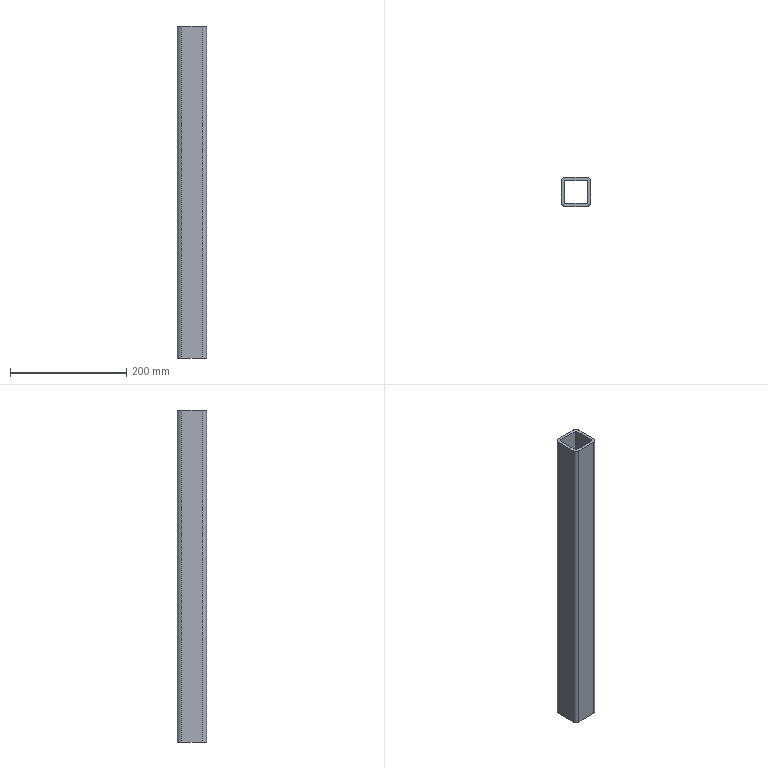Part | NX | 1 solid | 18 faces | box 50 x 50 x 570 mm | volume 490982 mm3 | plane 10 | cylinder 8 | commonest cylinder face diameters 4 x4 14 x4
STEP:
#1=CARTESIAN_POINT('',(-645.,-18.,285.));
#2=VERTEX_POINT('',#1);
#3=CARTESIAN_POINT('',(-645.,-18.,-285.));
#4=VERTEX_POINT('',#3);
#5=CARTESIAN_POINT('',(-645.,-18.,310.));
#6=DIRECTION('',(0.,0.,-1.));
#7=VECTOR('',#6,1000.);
#8=LINE('',#5,#7);
#9=EDGE_CURVE('',#2,#4,#8,.T.);
#10=ORIENTED_EDGE('',*,*,#9,.T.);
#11=CARTESIAN_POINT('',(-645.,18.,-285.));
#12=VERTEX_POINT('',#11);
#13=CARTESIAN_POINT('',(-645.,-18.,-285.));
#14=DIRECTION('',(0.,1.,0.));
#15=VECTOR('',#14,1000.);
#16=LINE('',#13,#15);
#17=EDGE_CURVE('',#4,#12,#16,.T.);
#18=ORIENTED_EDGE('',*,*,#17,.T.);
#19=CARTESIAN_POINT('',(-645.,18.,285.));
#20=VERTEX_POINT('',#19);
#21=CARTESIAN_POINT('',(-645.,18.,310.));
#22=DIRECTION('',(0.,0.,-1.));
#23=VECTOR('',#22,1000.);
#24=LINE('',#21,#23);
#25=EDGE_CURVE('',#20,#12,#24,.T.);
#26=ORIENTED_EDGE('',*,*,#25,.F.);
#27=CARTESIAN_POINT('',(-645.,-18.,285.));
#28=DIRECTION('',(0.,-1.,0.));
#29=VECTOR('',#28,1000.);
#30=LINE('',#27,#29);
#31=EDGE_CURVE('',#20,#2,#30,.T.);
#32=ORIENTED_EDGE('',*,*,#31,.T.);
#33=EDGE_LOOP('',(#10,#18,#26,#32));
#34=FACE_BOUND('',#33,.T.);
#35=CARTESIAN_POINT('',(-645.,-18.,310.));
#36=DIRECTION('',(1.,0.,0.));
#37=DIRECTION('',(0.,1.,0.));
#38=AXIS2_PLACEMENT_3D('',#35,#36,#37);
#39=PLANE('',#38);
#40=ADVANCED_FACE('',(#34),#39,.T.);
#41=CARTESIAN_POINT('',(-643.,-20.,285.));
#42=VERTEX_POINT('',#41);
#43=CARTESIAN_POINT('',(-643.,-20.,-285.));
#44=VERTEX_POINT('',#43);
#45=CARTESIAN_POINT('',(-643.,-20.,310.));
#46=DIRECTION('',(0.,0.,-1.));
#47=VECTOR('',#46,1000.);
#48=LINE('',#45,#47);
#49=EDGE_CURVE('',#42,#44,#48,.T.);
#50=ORIENTED_EDGE('',*,*,#49,.T.);
#51=CARTESIAN_POINT('',(-643.,-18.,-285.));
#52=DIRECTION('',(0.,0.,-1.));
#53=DIRECTION('',(-1.,0.,0.));
#54=AXIS2_PLACEMENT_3D('',#51,#52,#53);
#55=CIRCLE('',#54,2.);
#56=EDGE_CURVE('',#44,#4,#55,.T.);
#57=ORIENTED_EDGE('',*,*,#56,.T.);
#58=ORIENTED_EDGE('',*,*,#9,.F.);
#59=CARTESIAN_POINT('',(-643.,-18.,285.));
#60=DIRECTION('',(0.,0.,1.));
#61=DIRECTION('',(1.,0.,0.));
#62=AXIS2_PLACEMENT_3D('',#59,#60,#61);
#63=CIRCLE('',#62,2.);
#64=EDGE_CURVE('',#2,#42,#63,.T.);
#65=ORIENTED_EDGE('',*,*,#64,.T.);
#66=EDGE_LOOP('',(#50,#57,#58,#65));
#67=FACE_BOUND('',#66,.T.);
#68=CARTESIAN_POINT('',(-643.,-18.,310.));
#69=DIRECTION('',(0.,0.,-1.));
#70=DIRECTION('',(-1.,0.,0.));
#71=AXIS2_PLACEMENT_3D('',#68,#69,#70);
#72=CYLINDRICAL_SURFACE('',#71,2.);
#73=ADVANCED_FACE('',(#67),#72,.F.);
#74=CARTESIAN_POINT('',(-607.,-20.,285.));
#75=VERTEX_POINT('',#74);
#76=CARTESIAN_POINT('',(-607.,-20.,-285.));
#77=VERTEX_POINT('',#76);
#78=CARTESIAN_POINT('',(-607.,-20.,310.));
#79=DIRECTION('',(0.,0.,-1.));
#80=VECTOR('',#79,1000.);
#81=LINE('',#78,#80);
#82=EDGE_CURVE('',#75,#77,#81,.T.);
#83=ORIENTED_EDGE('',*,*,#82,.T.);
#84=CARTESIAN_POINT('',(-643.,-20.,-285.));
#85=DIRECTION('',(-1.,0.,0.));
#86=VECTOR('',#85,1000.);
#87=LINE('',#84,#86);
#88=EDGE_CURVE('',#77,#44,#87,.T.);
#89=ORIENTED_EDGE('',*,*,#88,.T.);
#90=ORIENTED_EDGE('',*,*,#49,.F.);
#91=CARTESIAN_POINT('',(-643.,-20.,285.));
#92=DIRECTION('',(1.,0.,0.));
#93=VECTOR('',#92,1000.);
#94=LINE('',#91,#93);
#95=EDGE_CURVE('',#42,#75,#94,.T.);
#96=ORIENTED_EDGE('',*,*,#95,.T.);
#97=EDGE_LOOP('',(#83,#89,#90,#96));
#98=FACE_BOUND('',#97,.T.);
#99=CARTESIAN_POINT('',(-643.,-20.,310.));
#100=DIRECTION('',(0.,1.,0.));
#101=DIRECTION('',(-1.,0.,0.));
#102=AXIS2_PLACEMENT_3D('',#99,#100,#101);
#103=PLANE('',#102);
#104=ADVANCED_FACE('',(#98),#103,.T.);
#105=CARTESIAN_POINT('',(-605.,-18.,285.));
#106=VERTEX_POINT('',#105);
#107=CARTESIAN_POINT('',(-605.,-18.,-285.));
#108=VERTEX_POINT('',#107);
#109=CARTESIAN_POINT('',(-605.,-18.,310.));
#110=DIRECTION('',(0.,0.,-1.));
#111=VECTOR('',#110,1000.);
#112=LINE('',#109,#111);
#113=EDGE_CURVE('',#106,#108,#112,.T.);
#114=ORIENTED_EDGE('',*,*,#113,.T.);
#115=CARTESIAN_POINT('',(-607.,-18.,-285.));
#116=DIRECTION('',(0.,0.,-1.));
#117=DIRECTION('',(-1.,0.,0.));
#118=AXIS2_PLACEMENT_3D('',#115,#116,#117);
#119=CIRCLE('',#118,2.);
#120=EDGE_CURVE('',#108,#77,#119,.T.);
#121=ORIENTED_EDGE('',*,*,#120,.T.);
#122=ORIENTED_EDGE('',*,*,#82,.F.);
#123=CARTESIAN_POINT('',(-607.,-18.,285.));
#124=DIRECTION('',(0.,0.,1.));
#125=DIRECTION('',(1.,0.,0.));
#126=AXIS2_PLACEMENT_3D('',#123,#124,#125);
#127=CIRCLE('',#126,2.);
#128=EDGE_CURVE('',#75,#106,#127,.T.);
#129=ORIENTED_EDGE('',*,*,#128,.T.);
#130=EDGE_LOOP('',(#114,#121,#122,#129));
#131=FACE_BOUND('',#130,.T.);
#132=CARTESIAN_POINT('',(-607.,-18.,310.));
#133=DIRECTION('',(0.,0.,-1.));
#134=DIRECTION('',(-1.,0.,0.));
#135=AXIS2_PLACEMENT_3D('',#132,#133,#134);
#136=CYLINDRICAL_SURFACE('',#135,2.);
#137=ADVANCED_FACE('',(#131),#136,.F.);
#138=CARTESIAN_POINT('',(-605.,18.,285.));
#139=VERTEX_POINT('',#138);
#140=CARTESIAN_POINT('',(-605.,18.,-285.));
#141=VERTEX_POINT('',#140);
#142=CARTESIAN_POINT('',(-605.,18.,310.));
#143=DIRECTION('',(0.,0.,-1.));
#144=VECTOR('',#143,1000.);
#145=LINE('',#142,#144);
#146=EDGE_CURVE('',#139,#141,#145,.T.);
#147=ORIENTED_EDGE('',*,*,#146,.T.);
#148=CARTESIAN_POINT('',(-605.,18.,-285.));
#149=DIRECTION('',(0.,-1.,0.));
#150=VECTOR('',#149,1000.);
#151=LINE('',#148,#150);
#152=EDGE_CURVE('',#141,#108,#151,.T.);
#153=ORIENTED_EDGE('',*,*,#152,.T.);
#154=ORIENTED_EDGE('',*,*,#113,.F.);
#155=CARTESIAN_POINT('',(-605.,18.,285.));
#156=DIRECTION('',(0.,1.,0.));
#157=VECTOR('',#156,1000.);
#158=LINE('',#155,#157);
#159=EDGE_CURVE('',#106,#139,#158,.T.);
#160=ORIENTED_EDGE('',*,*,#159,.T.);
#161=EDGE_LOOP('',(#147,#153,#154,#160));
#162=FACE_BOUND('',#161,.T.);
#163=CARTESIAN_POINT('',(-605.,18.,310.));
#164=DIRECTION('',(-1.,0.,0.));
#165=DIRECTION('',(0.,-1.,0.));
#166=AXIS2_PLACEMENT_3D('',#163,#164,#165);
#167=PLANE('',#166);
#168=ADVANCED_FACE('',(#162),#167,.T.);
#169=CARTESIAN_POINT('',(-607.,20.,285.));
#170=VERTEX_POINT('',#169);
#171=CARTESIAN_POINT('',(-607.,20.,-285.));
#172=VERTEX_POINT('',#171);
#173=CARTESIAN_POINT('',(-607.,20.,310.));
#174=DIRECTION('',(0.,0.,-1.));
#175=VECTOR('',#174,1000.);
#176=LINE('',#173,#175);
#177=EDGE_CURVE('',#170,#172,#176,.T.);
#178=ORIENTED_EDGE('',*,*,#177,.T.);
#179=CARTESIAN_POINT('',(-607.,18.,-285.));
#180=DIRECTION('',(0.,0.,-1.));
#181=DIRECTION('',(-1.,0.,0.));
#182=AXIS2_PLACEMENT_3D('',#179,#180,#181);
#183=CIRCLE('',#182,2.);
#184=EDGE_CURVE('',#172,#141,#183,.T.);
#185=ORIENTED_EDGE('',*,*,#184,.T.);
#186=ORIENTED_EDGE('',*,*,#146,.F.);
#187=CARTESIAN_POINT('',(-607.,18.,285.));
#188=DIRECTION('',(0.,0.,1.));
#189=DIRECTION('',(1.,0.,0.));
#190=AXIS2_PLACEMENT_3D('',#187,#188,#189);
#191=CIRCLE('',#190,2.);
#192=EDGE_CURVE('',#139,#170,#191,.T.);
#193=ORIENTED_EDGE('',*,*,#192,.T.);
#194=EDGE_LOOP('',(#178,#185,#186,#193));
#195=FACE_BOUND('',#194,.T.);
#196=CARTESIAN_POINT('',(-607.,18.,310.));
#197=DIRECTION('',(0.,0.,-1.));
#198=DIRECTION('',(-1.,0.,0.));
#199=AXIS2_PLACEMENT_3D('',#196,#197,#198);
#200=CYLINDRICAL_SURFACE('',#199,2.);
#201=ADVANCED_FACE('',(#195),#200,.F.);
#202=CARTESIAN_POINT('',(-643.,20.,285.));
#203=VERTEX_POINT('',#202);
#204=CARTESIAN_POINT('',(-643.,20.,-285.));
#205=VERTEX_POINT('',#204);
#206=CARTESIAN_POINT('',(-643.,20.,310.));
#207=DIRECTION('',(0.,0.,-1.));
#208=VECTOR('',#207,1000.);
#209=LINE('',#206,#208);
#210=EDGE_CURVE('',#203,#205,#209,.T.);
#211=ORIENTED_EDGE('',*,*,#210,.T.);
#212=CARTESIAN_POINT('',(-607.,20.,-285.));
#213=DIRECTION('',(1.,0.,0.));
#214=VECTOR('',#213,1000.);
#215=LINE('',#212,#214);
#216=EDGE_CURVE('',#205,#172,#215,.T.);
#217=ORIENTED_EDGE('',*,*,#216,.T.);
#218=ORIENTED_EDGE('',*,*,#177,.F.);
#219=CARTESIAN_POINT('',(-607.,20.,285.));
#220=DIRECTION('',(-1.,0.,0.));
#221=VECTOR('',#220,1000.);
#222=LINE('',#219,#221);
#223=EDGE_CURVE('',#170,#203,#222,.T.);
#224=ORIENTED_EDGE('',*,*,#223,.T.);
#225=EDGE_LOOP('',(#211,#217,#218,#224));
#226=FACE_BOUND('',#225,.T.);
#227=CARTESIAN_POINT('',(-607.,20.,310.));
#228=DIRECTION('',(0.,-1.,0.));
#229=DIRECTION('',(1.,0.,0.));
#230=AXIS2_PLACEMENT_3D('',#227,#228,#229);
#231=PLANE('',#230);
#232=ADVANCED_FACE('',(#226),#231,.T.);
#233=ORIENTED_EDGE('',*,*,#25,.T.);
#234=CARTESIAN_POINT('',(-643.,18.,-285.));
#235=DIRECTION('',(0.,0.,-1.));
#236=DIRECTION('',(-1.,0.,0.));
#237=AXIS2_PLACEMENT_3D('',#234,#235,#236);
#238=CIRCLE('',#237,2.);
#239=EDGE_CURVE('',#12,#205,#238,.T.);
#240=ORIENTED_EDGE('',*,*,#239,.T.);
#241=ORIENTED_EDGE('',*,*,#210,.F.);
#242=CARTESIAN_POINT('',(-643.,18.,285.));
#243=DIRECTION('',(0.,0.,1.));
#244=DIRECTION('',(1.,0.,0.));
#245=AXIS2_PLACEMENT_3D('',#242,#243,#244);
#246=CIRCLE('',#245,2.);
#247=EDGE_CURVE('',#203,#20,#246,.T.);
#248=ORIENTED_EDGE('',*,*,#247,.T.);
#249=EDGE_LOOP('',(#233,#240,#241,#248));
#250=FACE_BOUND('',#249,.T.);
#251=CARTESIAN_POINT('',(-643.,18.,310.));
#252=DIRECTION('',(0.,0.,-1.));
#253=DIRECTION('',(-1.,0.,0.));
#254=AXIS2_PLACEMENT_3D('',#251,#252,#253);
#255=CYLINDRICAL_SURFACE('',#254,2.);
#256=ADVANCED_FACE('',(#250),#255,.F.);
#257=CARTESIAN_POINT('',(-600.,18.,-285.));
#258=VERTEX_POINT('',#257);
#259=CARTESIAN_POINT('',(-600.,-18.,-285.));
#260=VERTEX_POINT('',#259);
#261=CARTESIAN_POINT('',(-600.,18.,-285.));
#262=DIRECTION('',(0.,-1.,0.));
#263=VECTOR('',#262,1000.);
#264=LINE('',#261,#263);
#265=EDGE_CURVE('',#258,#260,#264,.T.);
#266=ORIENTED_EDGE('',*,*,#265,.F.);
#267=CARTESIAN_POINT('',(-600.,18.,285.));
#268=VERTEX_POINT('',#267);
#269=CARTESIAN_POINT('',(-600.,18.,310.));
#270=DIRECTION('',(0.,0.,-1.));
#271=VECTOR('',#270,1000.);
#272=LINE('',#269,#271);
#273=EDGE_CURVE('',#268,#258,#272,.T.);
#274=ORIENTED_EDGE('',*,*,#273,.F.);
#275=CARTESIAN_POINT('',(-600.,-18.,285.));
#276=VERTEX_POINT('',#275);
#277=CARTESIAN_POINT('',(-600.,18.,285.));
#278=DIRECTION('',(0.,1.,0.));
#279=VECTOR('',#278,1000.);
#280=LINE('',#277,#279);
#281=EDGE_CURVE('',#276,#268,#280,.T.);
#282=ORIENTED_EDGE('',*,*,#281,.F.);
#283=CARTESIAN_POINT('',(-600.,-18.,310.));
#284=DIRECTION('',(0.,0.,-1.));
#285=VECTOR('',#284,1000.);
#286=LINE('',#283,#285);
#287=EDGE_CURVE('',#276,#260,#286,.T.);
#288=ORIENTED_EDGE('',*,*,#287,.T.);
#289=EDGE_LOOP('',(#266,#274,#282,#288));
#290=FACE_BOUND('',#289,.T.);
#291=CARTESIAN_POINT('',(-600.,18.,310.));
#292=DIRECTION('',(-1.,0.,0.));
#293=DIRECTION('',(0.,-1.,0.));
#294=AXIS2_PLACEMENT_3D('',#291,#292,#293);
#295=PLANE('',#294);
#296=ADVANCED_FACE('',(#290),#295,.F.);
#297=CARTESIAN_POINT('',(-607.,-25.,-285.));
#298=VERTEX_POINT('',#297);
#299=CARTESIAN_POINT('',(-607.,-18.,-285.));
#300=DIRECTION('',(0.,0.,-1.));
#301=DIRECTION('',(-1.,0.,0.));
#302=AXIS2_PLACEMENT_3D('',#299,#300,#301);
#303=CIRCLE('',#302,7.);
#304=EDGE_CURVE('',#260,#298,#303,.T.);
#305=ORIENTED_EDGE('',*,*,#304,.F.);
#306=ORIENTED_EDGE('',*,*,#287,.F.);
#307=CARTESIAN_POINT('',(-607.,-25.,285.));
#308=VERTEX_POINT('',#307);
#309=CARTESIAN_POINT('',(-607.,-18.,285.));
#310=DIRECTION('',(0.,0.,1.));
#311=DIRECTION('',(1.,0.,0.));
#312=AXIS2_PLACEMENT_3D('',#309,#310,#311);
#313=CIRCLE('',#312,7.);
#314=EDGE_CURVE('',#308,#276,#313,.T.);
#315=ORIENTED_EDGE('',*,*,#314,.F.);
#316=CARTESIAN_POINT('',(-607.,-25.,310.));
#317=DIRECTION('',(0.,0.,-1.));
#318=VECTOR('',#317,1000.);
#319=LINE('',#316,#318);
#320=EDGE_CURVE('',#308,#298,#319,.T.);
#321=ORIENTED_EDGE('',*,*,#320,.T.);
#322=EDGE_LOOP('',(#305,#306,#315,#321));
#323=FACE_BOUND('',#322,.T.);
#324=CARTESIAN_POINT('',(-607.,-18.,310.));
#325=DIRECTION('',(0.,0.,-1.));
#326=DIRECTION('',(-1.,0.,0.));
#327=AXIS2_PLACEMENT_3D('',#324,#325,#326);
#328=CYLINDRICAL_SURFACE('',#327,7.);
#329=ADVANCED_FACE('',(#323),#328,.T.);
#330=CARTESIAN_POINT('',(-643.,-25.,-285.));
#331=VERTEX_POINT('',#330);
#332=CARTESIAN_POINT('',(-875.,-25.,-285.));
#333=DIRECTION('',(1.,0.,0.));
#334=VECTOR('',#333,1000.);
#335=LINE('',#332,#334);
#336=EDGE_CURVE('',#331,#298,#335,.T.);
#337=ORIENTED_EDGE('',*,*,#336,.T.);
#338=ORIENTED_EDGE('',*,*,#320,.F.);
#339=CARTESIAN_POINT('',(-643.,-25.,285.));
#340=VERTEX_POINT('',#339);
#341=CARTESIAN_POINT('',(-875.,-25.,285.));
#342=DIRECTION('',(1.,0.,0.));
#343=VECTOR('',#342,1000.);
#344=LINE('',#341,#343);
#345=EDGE_CURVE('',#340,#308,#344,.T.);
#346=ORIENTED_EDGE('',*,*,#345,.F.);
#347=CARTESIAN_POINT('',(-643.,-25.,310.));
#348=DIRECTION('',(0.,0.,-1.));
#349=VECTOR('',#348,1000.);
#350=LINE('',#347,#349);
#351=EDGE_CURVE('',#340,#331,#350,.T.);
#352=ORIENTED_EDGE('',*,*,#351,.T.);
#353=EDGE_LOOP('',(#337,#338,#346,#352));
#354=FACE_BOUND('',#353,.T.);
#355=CARTESIAN_POINT('',(-643.,-25.,310.));
#356=DIRECTION('',(0.,1.,0.));
#357=DIRECTION('',(-1.,0.,0.));
#358=AXIS2_PLACEMENT_3D('',#355,#356,#357);
#359=PLANE('',#358);
#360=ADVANCED_FACE('',(#354),#359,.F.);
#361=CARTESIAN_POINT('',(-650.,-18.,-285.));
#362=VERTEX_POINT('',#361);
#363=CARTESIAN_POINT('',(-643.,-18.,-285.));
#364=DIRECTION('',(0.,0.,-1.));
#365=DIRECTION('',(-1.,0.,0.));
#366=AXIS2_PLACEMENT_3D('',#363,#364,#365);
#367=CIRCLE('',#366,7.);
#368=EDGE_CURVE('',#331,#362,#367,.T.);
#369=ORIENTED_EDGE('',*,*,#368,.F.);
#370=ORIENTED_EDGE('',*,*,#351,.F.);
#371=CARTESIAN_POINT('',(-650.,-18.,285.));
#372=VERTEX_POINT('',#371);
#373=CARTESIAN_POINT('',(-643.,-18.,285.));
#374=DIRECTION('',(0.,0.,1.));
#375=DIRECTION('',(1.,0.,0.));
#376=AXIS2_PLACEMENT_3D('',#373,#374,#375);
#377=CIRCLE('',#376,7.);
#378=EDGE_CURVE('',#372,#340,#377,.T.);
#379=ORIENTED_EDGE('',*,*,#378,.F.);
#380=CARTESIAN_POINT('',(-650.,-18.,310.));
#381=DIRECTION('',(0.,0.,-1.));
#382=VECTOR('',#381,1000.);
#383=LINE('',#380,#382);
#384=EDGE_CURVE('',#372,#362,#383,.T.);
#385=ORIENTED_EDGE('',*,*,#384,.T.);
#386=EDGE_LOOP('',(#369,#370,#379,#385));
#387=FACE_BOUND('',#386,.T.);
#388=CARTESIAN_POINT('',(-643.,-18.,310.));
#389=DIRECTION('',(0.,0.,-1.));
#390=DIRECTION('',(-1.,0.,0.));
#391=AXIS2_PLACEMENT_3D('',#388,#389,#390);
#392=CYLINDRICAL_SURFACE('',#391,7.);
#393=ADVANCED_FACE('',(#387),#392,.T.);
#394=CARTESIAN_POINT('',(-650.,18.,-285.));
#395=VERTEX_POINT('',#394);
#396=CARTESIAN_POINT('',(-650.,-18.,-285.));
#397=DIRECTION('',(0.,1.,0.));
#398=VECTOR('',#397,1000.);
#399=LINE('',#396,#398);
#400=EDGE_CURVE('',#362,#395,#399,.T.);
#401=ORIENTED_EDGE('',*,*,#400,.F.);
#402=ORIENTED_EDGE('',*,*,#384,.F.);
#403=CARTESIAN_POINT('',(-650.,18.,285.));
#404=VERTEX_POINT('',#403);
#405=CARTESIAN_POINT('',(-650.,-18.,285.));
#406=DIRECTION('',(0.,-1.,0.));
#407=VECTOR('',#406,1000.);
#408=LINE('',#405,#407);
#409=EDGE_CURVE('',#404,#372,#408,.T.);
#410=ORIENTED_EDGE('',*,*,#409,.F.);
#411=CARTESIAN_POINT('',(-650.,18.,310.));
#412=DIRECTION('',(0.,0.,-1.));
#413=VECTOR('',#412,1000.);
#414=LINE('',#411,#413);
#415=EDGE_CURVE('',#404,#395,#414,.T.);
#416=ORIENTED_EDGE('',*,*,#415,.T.);
#417=EDGE_LOOP('',(#401,#402,#410,#416));
#418=FACE_BOUND('',#417,.T.);
#419=CARTESIAN_POINT('',(-650.,-18.,310.));
#420=DIRECTION('',(1.,0.,0.));
#421=DIRECTION('',(0.,1.,0.));
#422=AXIS2_PLACEMENT_3D('',#419,#420,#421);
#423=PLANE('',#422);
#424=ADVANCED_FACE('',(#418),#423,.F.);
#425=CARTESIAN_POINT('',(-643.,25.,-285.));
#426=VERTEX_POINT('',#425);
#427=CARTESIAN_POINT('',(-643.,18.,-285.));
#428=DIRECTION('',(0.,0.,-1.));
#429=DIRECTION('',(-1.,0.,0.));
#430=AXIS2_PLACEMENT_3D('',#427,#428,#429);
#431=CIRCLE('',#430,7.);
#432=EDGE_CURVE('',#395,#426,#431,.T.);
#433=ORIENTED_EDGE('',*,*,#432,.F.);
#434=ORIENTED_EDGE('',*,*,#415,.F.);
#435=CARTESIAN_POINT('',(-643.,25.,285.));
#436=VERTEX_POINT('',#435);
#437=CARTESIAN_POINT('',(-643.,18.,285.));
#438=DIRECTION('',(0.,0.,1.));
#439=DIRECTION('',(1.,0.,0.));
#440=AXIS2_PLACEMENT_3D('',#437,#438,#439);
#441=CIRCLE('',#440,7.);
#442=EDGE_CURVE('',#436,#404,#441,.T.);
#443=ORIENTED_EDGE('',*,*,#442,.F.);
#444=CARTESIAN_POINT('',(-643.,25.,310.));
#445=DIRECTION('',(0.,0.,-1.));
#446=VECTOR('',#445,1000.);
#447=LINE('',#444,#446);
#448=EDGE_CURVE('',#436,#426,#447,.T.);
#449=ORIENTED_EDGE('',*,*,#448,.T.);
#450=EDGE_LOOP('',(#433,#434,#443,#449));
#451=FACE_BOUND('',#450,.T.);
#452=CARTESIAN_POINT('',(-643.,18.,310.));
#453=DIRECTION('',(0.,0.,-1.));
#454=DIRECTION('',(-1.,0.,0.));
#455=AXIS2_PLACEMENT_3D('',#452,#453,#454);
#456=CYLINDRICAL_SURFACE('',#455,7.);
#457=ADVANCED_FACE('',(#451),#456,.T.);
#458=CARTESIAN_POINT('',(-607.,25.,-285.));
#459=VERTEX_POINT('',#458);
#460=CARTESIAN_POINT('',(-875.,25.,-285.));
#461=DIRECTION('',(1.,0.,0.));
#462=VECTOR('',#461,1000.);
#463=LINE('',#460,#462);
#464=EDGE_CURVE('',#426,#459,#463,.T.);
#465=ORIENTED_EDGE('',*,*,#464,.F.);
#466=ORIENTED_EDGE('',*,*,#448,.F.);
#467=CARTESIAN_POINT('',(-607.,25.,285.));
#468=VERTEX_POINT('',#467);
#469=CARTESIAN_POINT('',(-875.,25.,285.));
#470=DIRECTION('',(1.,0.,0.));
#471=VECTOR('',#470,1000.);
#472=LINE('',#469,#471);
#473=EDGE_CURVE('',#436,#468,#472,.T.);
#474=ORIENTED_EDGE('',*,*,#473,.T.);
#475=CARTESIAN_POINT('',(-607.,25.,310.));
#476=DIRECTION('',(0.,0.,-1.));
#477=VECTOR('',#476,1000.);
#478=LINE('',#475,#477);
#479=EDGE_CURVE('',#468,#459,#478,.T.);
#480=ORIENTED_EDGE('',*,*,#479,.T.);
#481=EDGE_LOOP('',(#465,#466,#474,#480));
#482=FACE_BOUND('',#481,.T.);
#483=CARTESIAN_POINT('',(-607.,25.,310.));
#484=DIRECTION('',(0.,-1.,0.));
#485=DIRECTION('',(1.,0.,0.));
#486=AXIS2_PLACEMENT_3D('',#483,#484,#485);
#487=PLANE('',#486);
#488=ADVANCED_FACE('',(#482),#487,.F.);
#489=CARTESIAN_POINT('',(-607.,18.,-285.));
#490=DIRECTION('',(0.,0.,-1.));
#491=DIRECTION('',(-1.,0.,0.));
#492=AXIS2_PLACEMENT_3D('',#489,#490,#491);
#493=CIRCLE('',#492,7.);
#494=EDGE_CURVE('',#459,#258,#493,.T.);
#495=ORIENTED_EDGE('',*,*,#494,.F.);
#496=ORIENTED_EDGE('',*,*,#479,.F.);
#497=CARTESIAN_POINT('',(-607.,18.,285.));
#498=DIRECTION('',(0.,0.,1.));
#499=DIRECTION('',(1.,0.,0.));
#500=AXIS2_PLACEMENT_3D('',#497,#498,#499);
#501=CIRCLE('',#500,7.);
#502=EDGE_CURVE('',#268,#468,#501,.T.);
#503=ORIENTED_EDGE('',*,*,#502,.F.);
#504=ORIENTED_EDGE('',*,*,#273,.T.);
#505=EDGE_LOOP('',(#495,#496,#503,#504));
#506=FACE_BOUND('',#505,.T.);
#507=CARTESIAN_POINT('',(-607.,18.,310.));
#508=DIRECTION('',(0.,0.,-1.));
#509=DIRECTION('',(-1.,0.,0.));
#510=AXIS2_PLACEMENT_3D('',#507,#508,#509);
#511=CYLINDRICAL_SURFACE('',#510,7.);
#512=ADVANCED_FACE('',(#506),#511,.T.);
#513=ORIENTED_EDGE('',*,*,#223,.F.);
#514=ORIENTED_EDGE('',*,*,#192,.F.);
#515=ORIENTED_EDGE('',*,*,#159,.F.);
#516=ORIENTED_EDGE('',*,*,#128,.F.);
#517=ORIENTED_EDGE('',*,*,#95,.F.);
#518=ORIENTED_EDGE('',*,*,#64,.F.);
#519=ORIENTED_EDGE('',*,*,#31,.F.);
#520=ORIENTED_EDGE('',*,*,#247,.F.);
#521=EDGE_LOOP('',(#513,#514,#515,#516,#517,#518,#519,#520));
#522=FACE_BOUND('',#521,.T.);
#523=ORIENTED_EDGE('',*,*,#442,.T.);
#524=ORIENTED_EDGE('',*,*,#409,.T.);
#525=ORIENTED_EDGE('',*,*,#378,.T.);
#526=ORIENTED_EDGE('',*,*,#345,.T.);
#527=ORIENTED_EDGE('',*,*,#314,.T.);
#528=ORIENTED_EDGE('',*,*,#281,.T.);
#529=ORIENTED_EDGE('',*,*,#502,.T.);
#530=ORIENTED_EDGE('',*,*,#473,.F.);
#531=EDGE_LOOP('',(#523,#524,#525,#526,#527,#528,#529,#530));
#532=FACE_BOUND('',#531,.T.);
#533=CARTESIAN_POINT('',(-875.,-18.,285.));
#534=DIRECTION('',(0.,0.,1.));
#535=DIRECTION('',(1.,0.,0.));
#536=AXIS2_PLACEMENT_3D('',#533,#534,#535);
#537=PLANE('',#536);
#538=ADVANCED_FACE('',(#522,#532),#537,.T.);
#539=ORIENTED_EDGE('',*,*,#56,.F.);
#540=ORIENTED_EDGE('',*,*,#88,.F.);
#541=ORIENTED_EDGE('',*,*,#120,.F.);
#542=ORIENTED_EDGE('',*,*,#152,.F.);
#543=ORIENTED_EDGE('',*,*,#184,.F.);
#544=ORIENTED_EDGE('',*,*,#216,.F.);
#545=ORIENTED_EDGE('',*,*,#239,.F.);
#546=ORIENTED_EDGE('',*,*,#17,.F.);
#547=EDGE_LOOP('',(#539,#540,#541,#542,#543,#544,#545,#546));
#548=FACE_BOUND('',#547,.T.);
#549=ORIENTED_EDGE('',*,*,#368,.T.);
#550=ORIENTED_EDGE('',*,*,#400,.T.);
#551=ORIENTED_EDGE('',*,*,#432,.T.);
#552=ORIENTED_EDGE('',*,*,#464,.T.);
#553=ORIENTED_EDGE('',*,*,#494,.T.);
#554=ORIENTED_EDGE('',*,*,#265,.T.);
#555=ORIENTED_EDGE('',*,*,#304,.T.);
#556=ORIENTED_EDGE('',*,*,#336,.F.);
#557=EDGE_LOOP('',(#549,#550,#551,#552,#553,#554,#555,#556));
#558=FACE_BOUND('',#557,.T.);
#559=CARTESIAN_POINT('',(-875.,18.,-285.));
#560=DIRECTION('',(0.,0.,-1.));
#561=DIRECTION('',(-1.,0.,0.));
#562=AXIS2_PLACEMENT_3D('',#559,#560,#561);
#563=PLANE('',#562);
#564=ADVANCED_FACE('',(#548,#558),#563,.T.);
#565=CLOSED_SHELL('',(#40,#73,#104,#137,#168,#201,#232,#256,#296,#329,#360,#393,#424,#457,#488,#512,#538,#564));
#566=MANIFOLD_SOLID_BREP('',#565);
#567=(LENGTH_UNIT()NAMED_UNIT(*)SI_UNIT(.MILLI.,.METRE.));
#568=UNCERTAINTY_MEASURE_WITH_UNIT(LENGTH_MEASURE(0.00001),#567,'','');
#569=(NAMED_UNIT(*)PLANE_ANGLE_UNIT()SI_UNIT($,.RADIAN.));
#570=(NAMED_UNIT(*)SI_UNIT($,.STERADIAN.)SOLID_ANGLE_UNIT());
#571=(GEOMETRIC_REPRESENTATION_CONTEXT(3)GLOBAL_UNCERTAINTY_ASSIGNED_CONTEXT((#568))GLOBAL_UNIT_ASSIGNED_CONTEXT((#567,#569,#570))REPRESENTATION_CONTEXT('',''));
#572=ADVANCED_BREP_SHAPE_REPRESENTATION('',(#566),#571);